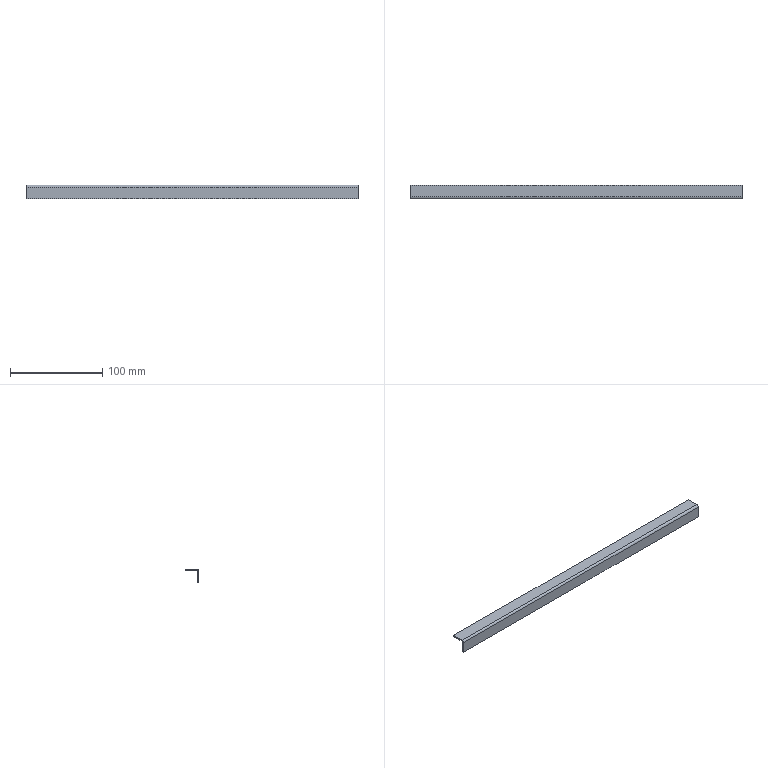Part | SolidWorks | features EdgeFlange 1, FlatPattern 1, SMBaseFlange 1, SheetMetal 1 | 1 solid | 14 faces | box 360 x 15 x 15 mm | volume 15045 mm3 | plane 12 | cylinder 2 | commonest cylinder face diameters 1.473 x1 4.473 x1
STEP:
#1=CARTESIAN_POINT('',(360.,-1.5,12.763));
#2=VERTEX_POINT('',#1);
#3=CARTESIAN_POINT('',(0.,-1.5,12.763));
#4=VERTEX_POINT('',#3);
#5=CARTESIAN_POINT('',(360.,-1.5,12.763));
#6=DIRECTION('',(-1.,0.,0.));
#7=VECTOR('',#6,1000.);
#8=LINE('',#5,#7);
#9=EDGE_CURVE('',#2,#4,#8,.T.);
#10=ORIENTED_EDGE('',*,*,#9,.T.);
#11=CARTESIAN_POINT('',(0.,-1.5,0.));
#12=VERTEX_POINT('',#11);
#13=CARTESIAN_POINT('',(0.,-1.5,15.));
#14=DIRECTION('',(0.,0.,-1.));
#15=VECTOR('',#14,1000.);
#16=LINE('',#13,#15);
#17=EDGE_CURVE('',#4,#12,#16,.T.);
#18=ORIENTED_EDGE('',*,*,#17,.T.);
#19=CARTESIAN_POINT('',(360.,-1.5,0.));
#20=VERTEX_POINT('',#19);
#21=CARTESIAN_POINT('',(0.,-1.5,0.));
#22=DIRECTION('',(1.,0.,0.));
#23=VECTOR('',#22,1000.);
#24=LINE('',#21,#23);
#25=EDGE_CURVE('',#12,#20,#24,.T.);
#26=ORIENTED_EDGE('',*,*,#25,.T.);
#27=CARTESIAN_POINT('',(360.,-1.5,15.));
#28=DIRECTION('',(0.,0.,-1.));
#29=VECTOR('',#28,1000.);
#30=LINE('',#27,#29);
#31=EDGE_CURVE('',#2,#20,#30,.T.);
#32=ORIENTED_EDGE('',*,*,#31,.F.);
#33=EDGE_LOOP('',(#10,#18,#26,#32));
#34=FACE_OUTER_BOUND('',#33,.T.);
#35=CARTESIAN_POINT('',(0.,-1.5,15.));
#36=DIRECTION('',(0.,1.,0.));
#37=DIRECTION('',(0.,0.,1.));
#38=AXIS2_PLACEMENT_3D('',#35,#36,#37);
#39=PLANE('',#38);
#40=ADVANCED_FACE('',(#34),#39,.F.);
#41=CARTESIAN_POINT('',(360.,0.,12.763));
#42=VERTEX_POINT('',#41);
#43=CARTESIAN_POINT('',(360.,0.,0.));
#44=VERTEX_POINT('',#43);
#45=CARTESIAN_POINT('',(360.,0.,15.));
#46=DIRECTION('',(0.,0.,-1.));
#47=VECTOR('',#46,1000.);
#48=LINE('',#45,#47);
#49=EDGE_CURVE('',#42,#44,#48,.T.);
#50=ORIENTED_EDGE('',*,*,#49,.F.);
#51=CARTESIAN_POINT('',(360.,0.,12.763));
#52=DIRECTION('',(0.,-1.,0.));
#53=VECTOR('',#52,1000.);
#54=LINE('',#51,#53);
#55=EDGE_CURVE('',#42,#2,#54,.T.);
#56=ORIENTED_EDGE('',*,*,#55,.T.);
#57=ORIENTED_EDGE('',*,*,#31,.T.);
#58=CARTESIAN_POINT('',(360.,0.,0.));
#59=DIRECTION('',(0.,-1.,0.));
#60=VECTOR('',#59,1000.);
#61=LINE('',#58,#60);
#62=EDGE_CURVE('',#44,#20,#61,.T.);
#63=ORIENTED_EDGE('',*,*,#62,.F.);
#64=EDGE_LOOP('',(#50,#56,#57,#63));
#65=FACE_OUTER_BOUND('',#64,.T.);
#66=CARTESIAN_POINT('',(360.,0.,15.));
#67=DIRECTION('',(1.,0.,0.));
#68=DIRECTION('',(0.,0.,-1.));
#69=AXIS2_PLACEMENT_3D('',#66,#67,#68);
#70=PLANE('',#69);
#71=ADVANCED_FACE('',(#65),#70,.T.);
#72=CARTESIAN_POINT('',(0.,0.,12.763));
#73=VERTEX_POINT('',#72);
#74=CARTESIAN_POINT('',(0.,0.,0.));
#75=VERTEX_POINT('',#74);
#76=CARTESIAN_POINT('',(0.,0.,15.));
#77=DIRECTION('',(0.,0.,-1.));
#78=VECTOR('',#77,1000.);
#79=LINE('',#76,#78);
#80=EDGE_CURVE('',#73,#75,#79,.T.);
#81=ORIENTED_EDGE('',*,*,#80,.F.);
#82=CARTESIAN_POINT('',(360.,0.,12.763));
#83=DIRECTION('',(-1.,0.,0.));
#84=VECTOR('',#83,1000.);
#85=LINE('',#82,#84);
#86=EDGE_CURVE('',#42,#73,#85,.T.);
#87=ORIENTED_EDGE('',*,*,#86,.F.);
#88=ORIENTED_EDGE('',*,*,#49,.T.);
#89=CARTESIAN_POINT('',(0.,0.,0.));
#90=DIRECTION('',(1.,0.,0.));
#91=VECTOR('',#90,1000.);
#92=LINE('',#89,#91);
#93=EDGE_CURVE('',#75,#44,#92,.T.);
#94=ORIENTED_EDGE('',*,*,#93,.F.);
#95=EDGE_LOOP('',(#81,#87,#88,#94));
#96=FACE_OUTER_BOUND('',#95,.T.);
#97=CARTESIAN_POINT('',(0.,0.,15.));
#98=DIRECTION('',(0.,1.,0.));
#99=DIRECTION('',(0.,0.,1.));
#100=AXIS2_PLACEMENT_3D('',#97,#98,#99);
#101=PLANE('',#100);
#102=ADVANCED_FACE('',(#96),#101,.T.);
#103=CARTESIAN_POINT('',(0.,0.,12.763));
#104=DIRECTION('',(0.,-1.,0.));
#105=VECTOR('',#104,1000.);
#106=LINE('',#103,#105);
#107=EDGE_CURVE('',#73,#4,#106,.T.);
#108=ORIENTED_EDGE('',*,*,#107,.F.);
#109=ORIENTED_EDGE('',*,*,#80,.T.);
#110=CARTESIAN_POINT('',(0.,-1.5,0.));
#111=DIRECTION('',(0.,1.,0.));
#112=VECTOR('',#111,1000.);
#113=LINE('',#110,#112);
#114=EDGE_CURVE('',#12,#75,#113,.T.);
#115=ORIENTED_EDGE('',*,*,#114,.F.);
#116=ORIENTED_EDGE('',*,*,#17,.F.);
#117=EDGE_LOOP('',(#108,#109,#115,#116));
#118=FACE_OUTER_BOUND('',#117,.T.);
#119=CARTESIAN_POINT('',(0.,-1.5,15.));
#120=DIRECTION('',(-1.,0.,0.));
#121=DIRECTION('',(0.,0.,1.));
#122=AXIS2_PLACEMENT_3D('',#119,#120,#121);
#123=PLANE('',#122);
#124=ADVANCED_FACE('',(#118),#123,.T.);
#125=ORIENTED_EDGE('',*,*,#25,.F.);
#126=ORIENTED_EDGE('',*,*,#114,.T.);
#127=ORIENTED_EDGE('',*,*,#93,.T.);
#128=ORIENTED_EDGE('',*,*,#62,.T.);
#129=EDGE_LOOP('',(#125,#126,#127,#128));
#130=FACE_OUTER_BOUND('',#129,.T.);
#131=CARTESIAN_POINT('',(0.,0.,0.));
#132=DIRECTION('',(0.,0.,-1.));
#133=DIRECTION('',(-1.,0.,0.));
#134=AXIS2_PLACEMENT_3D('',#131,#132,#133);
#135=PLANE('',#134);
#136=ADVANCED_FACE('',(#130),#135,.T.);
#137=CARTESIAN_POINT('',(0.,0.7366,13.5));
#138=VERTEX_POINT('',#137);
#139=CARTESIAN_POINT('',(0.,0.7366,15.));
#140=VERTEX_POINT('',#139);
#141=CARTESIAN_POINT('',(0.,0.7366,15.));
#142=DIRECTION('',(0.,0.,1.));
#143=VECTOR('',#142,1000.);
#144=LINE('',#141,#143);
#145=EDGE_CURVE('',#138,#140,#144,.T.);
#146=ORIENTED_EDGE('',*,*,#145,.F.);
#147=CARTESIAN_POINT('',(0.,0.7366,12.763));
#148=DIRECTION('',(-1.,0.,0.));
#149=DIRECTION('',(0.,0.,-1.));
#150=AXIS2_PLACEMENT_3D('',#147,#148,#149);
#151=CIRCLE('',#150,0.7366);
#152=EDGE_CURVE('',#73,#138,#151,.T.);
#153=ORIENTED_EDGE('',*,*,#152,.F.);
#154=ORIENTED_EDGE('',*,*,#107,.T.);
#155=CARTESIAN_POINT('',(0.,0.7366,12.763));
#156=DIRECTION('',(-1.,0.,0.));
#157=DIRECTION('',(0.,0.,-1.));
#158=AXIS2_PLACEMENT_3D('',#155,#156,#157);
#159=CIRCLE('',#158,2.237);
#160=EDGE_CURVE('',#4,#140,#159,.T.);
#161=ORIENTED_EDGE('',*,*,#160,.T.);
#162=EDGE_LOOP('',(#146,#153,#154,#161));
#163=FACE_OUTER_BOUND('',#162,.T.);
#164=CARTESIAN_POINT('',(0.,0.7366,12.763));
#165=DIRECTION('',(-1.,0.,0.));
#166=DIRECTION('',(0.,0.,1.));
#167=AXIS2_PLACEMENT_3D('',#164,#165,#166);
#168=PLANE('',#167);
#169=ADVANCED_FACE('',(#163),#168,.T.);
#170=CARTESIAN_POINT('',(360.,0.7366,13.5));
#171=VERTEX_POINT('',#170);
#172=CARTESIAN_POINT('',(360.,0.7366,12.763));
#173=DIRECTION('',(1.,0.,0.));
#174=DIRECTION('',(0.,0.,-1.));
#175=AXIS2_PLACEMENT_3D('',#172,#173,#174);
#176=CIRCLE('',#175,0.7366);
#177=EDGE_CURVE('',#171,#42,#176,.T.);
#178=ORIENTED_EDGE('',*,*,#177,.F.);
#179=CARTESIAN_POINT('',(360.,0.7366,15.));
#180=VERTEX_POINT('',#179);
#181=CARTESIAN_POINT('',(360.,0.7366,13.5));
#182=DIRECTION('',(0.,0.,1.));
#183=VECTOR('',#182,1000.);
#184=LINE('',#181,#183);
#185=EDGE_CURVE('',#171,#180,#184,.T.);
#186=ORIENTED_EDGE('',*,*,#185,.T.);
#187=CARTESIAN_POINT('',(360.,0.7366,12.763));
#188=DIRECTION('',(1.,0.,0.));
#189=DIRECTION('',(0.,0.,-1.));
#190=AXIS2_PLACEMENT_3D('',#187,#188,#189);
#191=CIRCLE('',#190,2.237);
#192=EDGE_CURVE('',#180,#2,#191,.T.);
#193=ORIENTED_EDGE('',*,*,#192,.T.);
#194=ORIENTED_EDGE('',*,*,#55,.F.);
#195=EDGE_LOOP('',(#178,#186,#193,#194));
#196=FACE_OUTER_BOUND('',#195,.T.);
#197=CARTESIAN_POINT('',(360.,0.7366,12.763));
#198=DIRECTION('',(-1.,0.,0.));
#199=DIRECTION('',(0.,0.,1.));
#200=AXIS2_PLACEMENT_3D('',#197,#198,#199);
#201=PLANE('',#200);
#202=ADVANCED_FACE('',(#196),#201,.F.);
#203=ORIENTED_EDGE('',*,*,#9,.F.);
#204=ORIENTED_EDGE('',*,*,#192,.F.);
#205=CARTESIAN_POINT('',(0.,0.7366,15.));
#206=DIRECTION('',(-1.,0.,0.));
#207=VECTOR('',#206,1000.);
#208=LINE('',#205,#207);
#209=EDGE_CURVE('',#180,#140,#208,.T.);
#210=ORIENTED_EDGE('',*,*,#209,.T.);
#211=ORIENTED_EDGE('',*,*,#160,.F.);
#212=EDGE_LOOP('',(#203,#204,#210,#211));
#213=FACE_OUTER_BOUND('',#212,.T.);
#214=CARTESIAN_POINT('',(360.,0.7366,12.763));
#215=DIRECTION('',(1.,0.,0.));
#216=DIRECTION('',(0.,0.,1.));
#217=AXIS2_PLACEMENT_3D('',#214,#215,#216);
#218=CYLINDRICAL_SURFACE('',#217,2.237);
#219=ADVANCED_FACE('',(#213),#218,.T.);
#220=ORIENTED_EDGE('',*,*,#86,.T.);
#221=ORIENTED_EDGE('',*,*,#152,.T.);
#222=CARTESIAN_POINT('',(0.,0.7366,13.5));
#223=DIRECTION('',(1.,0.,0.));
#224=VECTOR('',#223,1000.);
#225=LINE('',#222,#224);
#226=EDGE_CURVE('',#138,#171,#225,.T.);
#227=ORIENTED_EDGE('',*,*,#226,.T.);
#228=ORIENTED_EDGE('',*,*,#177,.T.);
#229=EDGE_LOOP('',(#220,#221,#227,#228));
#230=FACE_OUTER_BOUND('',#229,.T.);
#231=CARTESIAN_POINT('',(360.,0.7366,12.763));
#232=DIRECTION('',(1.,0.,0.));
#233=DIRECTION('',(0.,0.,1.));
#234=AXIS2_PLACEMENT_3D('',#231,#232,#233);
#235=CYLINDRICAL_SURFACE('',#234,0.7366);
#236=ADVANCED_FACE('',(#230),#235,.F.);
#237=ORIENTED_EDGE('',*,*,#145,.T.);
#238=CARTESIAN_POINT('',(0.,13.5,15.));
#239=VERTEX_POINT('',#238);
#240=CARTESIAN_POINT('',(0.,0.,15.));
#241=DIRECTION('',(0.,-1.,0.));
#242=VECTOR('',#241,1000.);
#243=LINE('',#240,#242);
#244=EDGE_CURVE('',#239,#140,#243,.T.);
#245=ORIENTED_EDGE('',*,*,#244,.F.);
#246=CARTESIAN_POINT('',(0.,13.5,13.5));
#247=VERTEX_POINT('',#246);
#248=CARTESIAN_POINT('',(0.,13.5,15.));
#249=DIRECTION('',(0.,0.,-1.));
#250=VECTOR('',#249,1000.);
#251=LINE('',#248,#250);
#252=EDGE_CURVE('',#239,#247,#251,.T.);
#253=ORIENTED_EDGE('',*,*,#252,.T.);
#254=CARTESIAN_POINT('',(0.,0.,13.5));
#255=DIRECTION('',(0.,-1.,0.));
#256=VECTOR('',#255,1000.);
#257=LINE('',#254,#256);
#258=EDGE_CURVE('',#247,#138,#257,.T.);
#259=ORIENTED_EDGE('',*,*,#258,.T.);
#260=EDGE_LOOP('',(#237,#245,#253,#259));
#261=FACE_OUTER_BOUND('',#260,.T.);
#262=CARTESIAN_POINT('',(0.,0.,15.));
#263=DIRECTION('',(1.,0.,0.));
#264=DIRECTION('',(0.,0.,-1.));
#265=AXIS2_PLACEMENT_3D('',#262,#263,#264);
#266=PLANE('',#265);
#267=ADVANCED_FACE('',(#261),#266,.F.);
#268=ORIENTED_EDGE('',*,*,#185,.F.);
#269=CARTESIAN_POINT('',(360.,13.5,13.5));
#270=VERTEX_POINT('',#269);
#271=CARTESIAN_POINT('',(360.,13.5,13.5));
#272=DIRECTION('',(0.,1.,0.));
#273=VECTOR('',#272,1000.);
#274=LINE('',#271,#273);
#275=EDGE_CURVE('',#171,#270,#274,.T.);
#276=ORIENTED_EDGE('',*,*,#275,.T.);
#277=CARTESIAN_POINT('',(360.,13.5,15.));
#278=VERTEX_POINT('',#277);
#279=CARTESIAN_POINT('',(360.,13.5,15.));
#280=DIRECTION('',(0.,0.,-1.));
#281=VECTOR('',#280,1000.);
#282=LINE('',#279,#281);
#283=EDGE_CURVE('',#278,#270,#282,.T.);
#284=ORIENTED_EDGE('',*,*,#283,.F.);
#285=CARTESIAN_POINT('',(360.,0.,15.));
#286=DIRECTION('',(0.,1.,0.));
#287=VECTOR('',#286,1000.);
#288=LINE('',#285,#287);
#289=EDGE_CURVE('',#180,#278,#288,.T.);
#290=ORIENTED_EDGE('',*,*,#289,.F.);
#291=EDGE_LOOP('',(#268,#276,#284,#290));
#292=FACE_OUTER_BOUND('',#291,.T.);
#293=CARTESIAN_POINT('',(360.,13.5,15.));
#294=DIRECTION('',(-1.,0.,0.));
#295=DIRECTION('',(0.,0.,1.));
#296=AXIS2_PLACEMENT_3D('',#293,#294,#295);
#297=PLANE('',#296);
#298=ADVANCED_FACE('',(#292),#297,.F.);
#299=ORIENTED_EDGE('',*,*,#209,.F.);
#300=ORIENTED_EDGE('',*,*,#289,.T.);
#301=CARTESIAN_POINT('',(0.,13.5,15.));
#302=DIRECTION('',(-1.,0.,0.));
#303=VECTOR('',#302,1000.);
#304=LINE('',#301,#303);
#305=EDGE_CURVE('',#278,#239,#304,.T.);
#306=ORIENTED_EDGE('',*,*,#305,.T.);
#307=ORIENTED_EDGE('',*,*,#244,.T.);
#308=EDGE_LOOP('',(#299,#300,#306,#307));
#309=FACE_OUTER_BOUND('',#308,.T.);
#310=CARTESIAN_POINT('',(0.,0.,15.));
#311=DIRECTION('',(0.,0.,-1.));
#312=DIRECTION('',(-1.,0.,0.));
#313=AXIS2_PLACEMENT_3D('',#310,#311,#312);
#314=PLANE('',#313);
#315=ADVANCED_FACE('',(#309),#314,.F.);
#316=ORIENTED_EDGE('',*,*,#275,.F.);
#317=ORIENTED_EDGE('',*,*,#226,.F.);
#318=ORIENTED_EDGE('',*,*,#258,.F.);
#319=CARTESIAN_POINT('',(0.,13.5,13.5));
#320=DIRECTION('',(-1.,0.,0.));
#321=VECTOR('',#320,1000.);
#322=LINE('',#319,#321);
#323=EDGE_CURVE('',#270,#247,#322,.T.);
#324=ORIENTED_EDGE('',*,*,#323,.F.);
#325=EDGE_LOOP('',(#316,#317,#318,#324));
#326=FACE_OUTER_BOUND('',#325,.T.);
#327=CARTESIAN_POINT('',(0.,0.,13.5));
#328=DIRECTION('',(0.,0.,-1.));
#329=DIRECTION('',(-1.,0.,0.));
#330=AXIS2_PLACEMENT_3D('',#327,#328,#329);
#331=PLANE('',#330);
#332=ADVANCED_FACE('',(#326),#331,.T.);
#333=ORIENTED_EDGE('',*,*,#323,.T.);
#334=ORIENTED_EDGE('',*,*,#252,.F.);
#335=ORIENTED_EDGE('',*,*,#305,.F.);
#336=ORIENTED_EDGE('',*,*,#283,.T.);
#337=EDGE_LOOP('',(#333,#334,#335,#336));
#338=FACE_OUTER_BOUND('',#337,.T.);
#339=CARTESIAN_POINT('',(0.,13.5,15.));
#340=DIRECTION('',(0.,-1.,0.));
#341=DIRECTION('',(0.,0.,-1.));
#342=AXIS2_PLACEMENT_3D('',#339,#340,#341);
#343=PLANE('',#342);
#344=ADVANCED_FACE('',(#338),#343,.F.);
#345=CLOSED_SHELL('',(#40,#71,#102,#124,#136,#169,#202,#219,#236,#267,#298,#315,#332,#344));
#346=MANIFOLD_SOLID_BREP('',#345);
#347=CARTESIAN_POINT('',(0.,0.,0.));
#348=DIRECTION('',(0.,0.,1.));
#349=DIRECTION('',(1.,0.,0.));
#350=AXIS2_PLACEMENT_3D('',#347,#348,#349);
#351=(LENGTH_UNIT()NAMED_UNIT(*)SI_UNIT(.MILLI.,.METRE.));
#352=UNCERTAINTY_MEASURE_WITH_UNIT(LENGTH_MEASURE(0.00001),#351,'','');
#353=(NAMED_UNIT(*)PLANE_ANGLE_UNIT()SI_UNIT($,.RADIAN.));
#354=(NAMED_UNIT(*)SI_UNIT($,.STERADIAN.)SOLID_ANGLE_UNIT());
#355=(GEOMETRIC_REPRESENTATION_CONTEXT(3)GLOBAL_UNCERTAINTY_ASSIGNED_CONTEXT((#352))GLOBAL_UNIT_ASSIGNED_CONTEXT((#351,#353,#354))REPRESENTATION_CONTEXT('',''));
#356=ADVANCED_BREP_SHAPE_REPRESENTATION('',(#346,#350),#355);